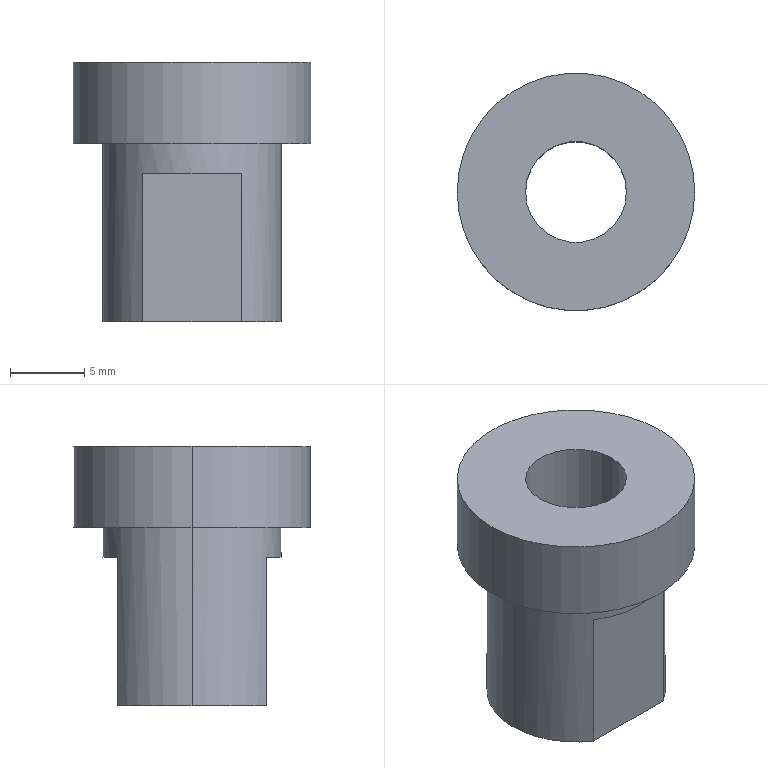Part | STEP file | 2029 Bag feed cylinder joint | 1 solid | 13 faces | box 16 x 16 x 17.5 mm | volume 1737 mm3 | plane 7 | cylinder 6 | commonest cylinder face diameters 6.8 x2 12 x2 16 x2
STEP:
#1=CARTESIAN_POINT('',(0.,0.,0.));
#2=DIRECTION('',(0.,0.,1.));
#3=DIRECTION('',(1.,0.,0.));
#4=AXIS2_PLACEMENT_3D('',#1,#2,#3);
#5=CARTESIAN_POINT('',(-3.4,0.,17.5));
#6=VERTEX_POINT('',#5);
#7=CARTESIAN_POINT('',(-3.4,0.,0.));
#8=VERTEX_POINT('',#7);
#9=CARTESIAN_POINT('',(-3.4,0.,0.));
#10=DIRECTION('',(0.,0.,-1.));
#11=VECTOR('',#10,1.);
#12=LINE('',#9,#11);
#13=CARTESIAN_POINT('',(0.,0.,0.));
#14=DIRECTION('',(0.,0.,-1.));
#15=DIRECTION('',(-1.,0.,0.));
#16=AXIS2_PLACEMENT_3D('',#13,#14,#15);
#17=CYLINDRICAL_SURFACE('',#16,3.4);
#18=CARTESIAN_POINT('',(6.283,0.));
#19=DIRECTION('',(0.,1.));
#20=VECTOR('',#19,1.);
#21=LINE('',#18,#20);
#22=(GEOMETRIC_REPRESENTATION_CONTEXT(2)PARAMETRIC_REPRESENTATION_CONTEXT()REPRESENTATION_CONTEXT('',''));
#23=DEFINITIONAL_REPRESENTATION('',(#21),#22);
#24=PCURVE('',#17,#23);
#25=CARTESIAN_POINT('',(0.,0.,0.));
#26=DIRECTION('',(0.,0.,-1.));
#27=DIRECTION('',(-1.,0.,0.));
#28=AXIS2_PLACEMENT_3D('',#25,#26,#27);
#29=CYLINDRICAL_SURFACE('',#28,3.4);
#30=CARTESIAN_POINT('',(0.,0.));
#31=DIRECTION('',(0.,1.));
#32=VECTOR('',#31,1.);
#33=LINE('',#30,#32);
#34=(GEOMETRIC_REPRESENTATION_CONTEXT(2)PARAMETRIC_REPRESENTATION_CONTEXT()REPRESENTATION_CONTEXT('',''));
#35=DEFINITIONAL_REPRESENTATION('',(#33),#34);
#36=PCURVE('',#29,#35);
#37=SURFACE_CURVE('',#12,(#24,#36),.PCURVE_S1.);
#38=EDGE_CURVE('',#6,#8,#37,.T.);
#39=ORIENTED_EDGE('',*,*,#38,.T.);
#40=CARTESIAN_POINT('',(3.4,0.,0.));
#41=VERTEX_POINT('',#40);
#42=CARTESIAN_POINT('',(0.,0.,0.));
#43=DIRECTION('',(0.,0.,-1.));
#44=DIRECTION('',(-1.,0.,0.));
#45=AXIS2_PLACEMENT_3D('',#42,#43,#44);
#46=CIRCLE('',#45,3.4);
#47=CARTESIAN_POINT('',(0.,0.));
#48=DIRECTION('',(1.,0.));
#49=VECTOR('',#48,1.);
#50=LINE('',#47,#49);
#51=(GEOMETRIC_REPRESENTATION_CONTEXT(2)PARAMETRIC_REPRESENTATION_CONTEXT()REPRESENTATION_CONTEXT('',''));
#52=DEFINITIONAL_REPRESENTATION('',(#50),#51);
#53=PCURVE('',#17,#52);
#54=CARTESIAN_POINT('',(0.,0.,0.));
#55=DIRECTION('',(0.,0.,1.));
#56=DIRECTION('',(1.,0.,0.));
#57=AXIS2_PLACEMENT_3D('',#54,#55,#56);
#58=PLANE('',#57);
#59=CARTESIAN_POINT('',(-3.4,0.));
#60=CARTESIAN_POINT('',(-3.4,5.889));
#61=CARTESIAN_POINT('',(1.7,2.944));
#62=CARTESIAN_POINT('',(6.8,0.));
#63=CARTESIAN_POINT('',(1.7,-2.944));
#64=CARTESIAN_POINT('',(-3.4,-5.889));
#65=CARTESIAN_POINT('',(-3.4,0.));
#66=(BOUNDED_CURVE()B_SPLINE_CURVE(2,(#59,#60,#61,#62,#63,#64,#65),.UNSPECIFIED.,.T.,.F.)B_SPLINE_CURVE_WITH_KNOTS((1,2,2,2,2,1),(-2.094,0.,2.094,4.189,6.283,8.378),.UNSPECIFIED.)CURVE()GEOMETRIC_REPRESENTATION_ITEM()RATIONAL_B_SPLINE_CURVE((1.,0.5,1.,0.5,1.,0.5,1.))REPRESENTATION_ITEM(''));
#67=(GEOMETRIC_REPRESENTATION_CONTEXT(2)PARAMETRIC_REPRESENTATION_CONTEXT()REPRESENTATION_CONTEXT('',''));
#68=DEFINITIONAL_REPRESENTATION('',(#66),#67);
#69=PCURVE('',#58,#68);
#70=SURFACE_CURVE('',#46,(#53,#69),.PCURVE_S1.);
#71=EDGE_CURVE('',#41,#8,#70,.T.);
#72=ORIENTED_EDGE('',*,*,#71,.F.);
#73=CARTESIAN_POINT('',(3.4,0.,17.5));
#74=VERTEX_POINT('',#73);
#75=CARTESIAN_POINT('',(3.4,0.,0.));
#76=DIRECTION('',(0.,0.,-1.));
#77=VECTOR('',#76,1.);
#78=LINE('',#75,#77);
#79=CARTESIAN_POINT('',(3.142,0.));
#80=DIRECTION('',(0.,1.));
#81=VECTOR('',#80,1.);
#82=LINE('',#79,#81);
#83=(GEOMETRIC_REPRESENTATION_CONTEXT(2)PARAMETRIC_REPRESENTATION_CONTEXT()REPRESENTATION_CONTEXT('',''));
#84=DEFINITIONAL_REPRESENTATION('',(#82),#83);
#85=PCURVE('',#17,#84);
#86=CARTESIAN_POINT('',(3.142,0.));
#87=DIRECTION('',(0.,1.));
#88=VECTOR('',#87,1.);
#89=LINE('',#86,#88);
#90=(GEOMETRIC_REPRESENTATION_CONTEXT(2)PARAMETRIC_REPRESENTATION_CONTEXT()REPRESENTATION_CONTEXT('',''));
#91=DEFINITIONAL_REPRESENTATION('',(#89),#90);
#92=PCURVE('',#29,#91);
#93=SURFACE_CURVE('',#78,(#85,#92),.PCURVE_S1.);
#94=EDGE_CURVE('',#74,#41,#93,.T.);
#95=ORIENTED_EDGE('',*,*,#94,.F.);
#96=CARTESIAN_POINT('',(0.,0.,17.5));
#97=DIRECTION('',(0.,0.,-1.));
#98=DIRECTION('',(-1.,0.,0.));
#99=AXIS2_PLACEMENT_3D('',#96,#97,#98);
#100=CIRCLE('',#99,3.4);
#101=CARTESIAN_POINT('',(0.,-17.5));
#102=DIRECTION('',(1.,0.));
#103=VECTOR('',#102,1.);
#104=LINE('',#101,#103);
#105=(GEOMETRIC_REPRESENTATION_CONTEXT(2)PARAMETRIC_REPRESENTATION_CONTEXT()REPRESENTATION_CONTEXT('',''));
#106=DEFINITIONAL_REPRESENTATION('',(#104),#105);
#107=PCURVE('',#17,#106);
#108=CARTESIAN_POINT('',(0.,0.,17.5));
#109=DIRECTION('',(0.,0.,1.));
#110=DIRECTION('',(1.,0.,0.));
#111=AXIS2_PLACEMENT_3D('',#108,#109,#110);
#112=PLANE('',#111);
#113=CARTESIAN_POINT('',(-3.4,0.));
#114=CARTESIAN_POINT('',(-3.4,5.889));
#115=CARTESIAN_POINT('',(1.7,2.944));
#116=CARTESIAN_POINT('',(6.8,0.));
#117=CARTESIAN_POINT('',(1.7,-2.944));
#118=CARTESIAN_POINT('',(-3.4,-5.889));
#119=CARTESIAN_POINT('',(-3.4,0.));
#120=(BOUNDED_CURVE()B_SPLINE_CURVE(2,(#113,#114,#115,#116,#117,#118,#119),.UNSPECIFIED.,.T.,.F.)B_SPLINE_CURVE_WITH_KNOTS((1,2,2,2,2,1),(-2.094,0.,2.094,4.189,6.283,8.378),.UNSPECIFIED.)CURVE()GEOMETRIC_REPRESENTATION_ITEM()RATIONAL_B_SPLINE_CURVE((1.,0.5,1.,0.5,1.,0.5,1.))REPRESENTATION_ITEM(''));
#121=(GEOMETRIC_REPRESENTATION_CONTEXT(2)PARAMETRIC_REPRESENTATION_CONTEXT()REPRESENTATION_CONTEXT('',''));
#122=DEFINITIONAL_REPRESENTATION('',(#120),#121);
#123=PCURVE('',#112,#122);
#124=SURFACE_CURVE('',#100,(#107,#123),.PCURVE_S1.);
#125=EDGE_CURVE('',#74,#6,#124,.T.);
#126=ORIENTED_EDGE('',*,*,#125,.T.);
#127=EDGE_LOOP('',(#39,#72,#95,#126));
#128=FACE_BOUND('',#127,.F.);
#129=ADVANCED_FACE('',(#128),#17,.F.);
#130=CARTESIAN_POINT('',(8.,0.,17.5));
#131=VERTEX_POINT('',#130);
#132=CARTESIAN_POINT('',(-8.,0.,17.5));
#133=VERTEX_POINT('',#132);
#134=CARTESIAN_POINT('',(0.,0.,17.5));
#135=DIRECTION('',(0.,0.,1.));
#136=DIRECTION('',(1.,0.,0.));
#137=AXIS2_PLACEMENT_3D('',#134,#135,#136);
#138=CIRCLE('',#137,8.);
#139=CARTESIAN_POINT('',(0.,0.,17.5));
#140=DIRECTION('',(0.,0.,-1.));
#141=DIRECTION('',(-1.,0.,0.));
#142=AXIS2_PLACEMENT_3D('',#139,#140,#141);
#143=CYLINDRICAL_SURFACE('',#142,8.);
#144=CARTESIAN_POINT('',(3.142,0.));
#145=DIRECTION('',(-1.,0.));
#146=VECTOR('',#145,1.);
#147=LINE('',#144,#146);
#148=(GEOMETRIC_REPRESENTATION_CONTEXT(2)PARAMETRIC_REPRESENTATION_CONTEXT()REPRESENTATION_CONTEXT('',''));
#149=DEFINITIONAL_REPRESENTATION('',(#147),#148);
#150=PCURVE('',#143,#149);
#151=CARTESIAN_POINT('',(0.,0.));
#152=DIRECTION('',(1.,0.));
#153=AXIS2_PLACEMENT_2D('',#151,#152);
#154=CIRCLE('',#153,8.);
#155=(GEOMETRIC_REPRESENTATION_CONTEXT(2)PARAMETRIC_REPRESENTATION_CONTEXT()REPRESENTATION_CONTEXT('',''));
#156=DEFINITIONAL_REPRESENTATION('',(#154),#155);
#157=PCURVE('',#112,#156);
#158=SURFACE_CURVE('',#138,(#150,#157),.PCURVE_S1.);
#159=EDGE_CURVE('',#131,#133,#158,.T.);
#160=ORIENTED_EDGE('',*,*,#159,.F.);
#161=CARTESIAN_POINT('',(8.,0.,12.));
#162=VERTEX_POINT('',#161);
#163=CARTESIAN_POINT('',(8.,0.,17.5));
#164=DIRECTION('',(0.,0.,-1.));
#165=VECTOR('',#164,1.);
#166=LINE('',#163,#165);
#167=CARTESIAN_POINT('',(3.142,0.));
#168=DIRECTION('',(0.,1.));
#169=VECTOR('',#168,1.);
#170=LINE('',#167,#169);
#171=(GEOMETRIC_REPRESENTATION_CONTEXT(2)PARAMETRIC_REPRESENTATION_CONTEXT()REPRESENTATION_CONTEXT('',''));
#172=DEFINITIONAL_REPRESENTATION('',(#170),#171);
#173=PCURVE('',#143,#172);
#174=CARTESIAN_POINT('',(0.,0.,17.5));
#175=DIRECTION('',(0.,0.,-1.));
#176=DIRECTION('',(-1.,0.,0.));
#177=AXIS2_PLACEMENT_3D('',#174,#175,#176);
#178=CYLINDRICAL_SURFACE('',#177,8.);
#179=CARTESIAN_POINT('',(3.142,0.));
#180=DIRECTION('',(0.,1.));
#181=VECTOR('',#180,1.);
#182=LINE('',#179,#181);
#183=(GEOMETRIC_REPRESENTATION_CONTEXT(2)PARAMETRIC_REPRESENTATION_CONTEXT()REPRESENTATION_CONTEXT('',''));
#184=DEFINITIONAL_REPRESENTATION('',(#182),#183);
#185=PCURVE('',#178,#184);
#186=SURFACE_CURVE('',#166,(#173,#185),.PCURVE_S1.);
#187=EDGE_CURVE('',#131,#162,#186,.T.);
#188=ORIENTED_EDGE('',*,*,#187,.T.);
#189=CARTESIAN_POINT('',(-8.,0.,12.));
#190=VERTEX_POINT('',#189);
#191=CARTESIAN_POINT('',(0.,0.,12.));
#192=DIRECTION('',(0.,0.,1.));
#193=DIRECTION('',(1.,0.,0.));
#194=AXIS2_PLACEMENT_3D('',#191,#192,#193);
#195=CIRCLE('',#194,8.);
#196=CARTESIAN_POINT('',(3.142,5.5));
#197=DIRECTION('',(-1.,0.));
#198=VECTOR('',#197,1.);
#199=LINE('',#196,#198);
#200=(GEOMETRIC_REPRESENTATION_CONTEXT(2)PARAMETRIC_REPRESENTATION_CONTEXT()REPRESENTATION_CONTEXT('',''));
#201=DEFINITIONAL_REPRESENTATION('',(#199),#200);
#202=PCURVE('',#143,#201);
#203=CARTESIAN_POINT('',(0.,0.,12.));
#204=DIRECTION('',(0.,0.,1.));
#205=DIRECTION('',(1.,0.,0.));
#206=AXIS2_PLACEMENT_3D('',#203,#204,#205);
#207=PLANE('',#206);
#208=CARTESIAN_POINT('',(0.,0.));
#209=DIRECTION('',(1.,0.));
#210=AXIS2_PLACEMENT_2D('',#208,#209);
#211=CIRCLE('',#210,8.);
#212=(GEOMETRIC_REPRESENTATION_CONTEXT(2)PARAMETRIC_REPRESENTATION_CONTEXT()REPRESENTATION_CONTEXT('',''));
#213=DEFINITIONAL_REPRESENTATION('',(#211),#212);
#214=PCURVE('',#207,#213);
#215=SURFACE_CURVE('',#195,(#202,#214),.PCURVE_S1.);
#216=EDGE_CURVE('',#162,#190,#215,.T.);
#217=ORIENTED_EDGE('',*,*,#216,.T.);
#218=CARTESIAN_POINT('',(-8.,0.,17.5));
#219=DIRECTION('',(0.,0.,-1.));
#220=VECTOR('',#219,1.);
#221=LINE('',#218,#220);
#222=CARTESIAN_POINT('',(0.,0.));
#223=DIRECTION('',(0.,1.));
#224=VECTOR('',#223,1.);
#225=LINE('',#222,#224);
#226=(GEOMETRIC_REPRESENTATION_CONTEXT(2)PARAMETRIC_REPRESENTATION_CONTEXT()REPRESENTATION_CONTEXT('',''));
#227=DEFINITIONAL_REPRESENTATION('',(#225),#226);
#228=PCURVE('',#143,#227);
#229=CARTESIAN_POINT('',(6.283,0.));
#230=DIRECTION('',(0.,1.));
#231=VECTOR('',#230,1.);
#232=LINE('',#229,#231);
#233=(GEOMETRIC_REPRESENTATION_CONTEXT(2)PARAMETRIC_REPRESENTATION_CONTEXT()REPRESENTATION_CONTEXT('',''));
#234=DEFINITIONAL_REPRESENTATION('',(#232),#233);
#235=PCURVE('',#178,#234);
#236=SURFACE_CURVE('',#221,(#228,#235),.PCURVE_S1.);
#237=EDGE_CURVE('',#133,#190,#236,.T.);
#238=ORIENTED_EDGE('',*,*,#237,.F.);
#239=EDGE_LOOP('',(#160,#188,#217,#238));
#240=FACE_BOUND('',#239,.T.);
#241=ADVANCED_FACE('',(#240),#143,.T.);
#242=CARTESIAN_POINT('',(6.,0.,12.));
#243=VERTEX_POINT('',#242);
#244=CARTESIAN_POINT('',(-6.,0.,12.));
#245=VERTEX_POINT('',#244);
#246=CARTESIAN_POINT('',(0.,0.,12.));
#247=DIRECTION('',(0.,0.,1.));
#248=DIRECTION('',(1.,0.,0.));
#249=AXIS2_PLACEMENT_3D('',#246,#247,#248);
#250=CIRCLE('',#249,6.);
#251=CARTESIAN_POINT('',(0.,0.,12.));
#252=DIRECTION('',(0.,0.,-1.));
#253=DIRECTION('',(-1.,0.,0.));
#254=AXIS2_PLACEMENT_3D('',#251,#252,#253);
#255=CYLINDRICAL_SURFACE('',#254,6.);
#256=CARTESIAN_POINT('',(3.142,0.));
#257=DIRECTION('',(-1.,0.));
#258=VECTOR('',#257,1.);
#259=LINE('',#256,#258);
#260=(GEOMETRIC_REPRESENTATION_CONTEXT(2)PARAMETRIC_REPRESENTATION_CONTEXT()REPRESENTATION_CONTEXT('',''));
#261=DEFINITIONAL_REPRESENTATION('',(#259),#260);
#262=PCURVE('',#255,#261);
#263=CARTESIAN_POINT('',(0.,0.));
#264=DIRECTION('',(1.,0.));
#265=AXIS2_PLACEMENT_2D('',#263,#264);
#266=CIRCLE('',#265,6.);
#267=(GEOMETRIC_REPRESENTATION_CONTEXT(2)PARAMETRIC_REPRESENTATION_CONTEXT()REPRESENTATION_CONTEXT('',''));
#268=DEFINITIONAL_REPRESENTATION('',(#266),#267);
#269=PCURVE('',#207,#268);
#270=SURFACE_CURVE('',#250,(#262,#269),.PCURVE_S1.);
#271=EDGE_CURVE('',#243,#245,#270,.T.);
#272=ORIENTED_EDGE('',*,*,#271,.F.);
#273=CARTESIAN_POINT('',(6.,0.,0.));
#274=VERTEX_POINT('',#273);
#275=CARTESIAN_POINT('',(6.,0.,12.));
#276=DIRECTION('',(0.,0.,-1.));
#277=VECTOR('',#276,1.);
#278=LINE('',#275,#277);
#279=CARTESIAN_POINT('',(3.142,0.));
#280=DIRECTION('',(0.,1.));
#281=VECTOR('',#280,1.);
#282=LINE('',#279,#281);
#283=(GEOMETRIC_REPRESENTATION_CONTEXT(2)PARAMETRIC_REPRESENTATION_CONTEXT()REPRESENTATION_CONTEXT('',''));
#284=DEFINITIONAL_REPRESENTATION('',(#282),#283);
#285=PCURVE('',#255,#284);
#286=CARTESIAN_POINT('',(0.,0.,12.));
#287=DIRECTION('',(0.,0.,-1.));
#288=DIRECTION('',(-1.,0.,0.));
#289=AXIS2_PLACEMENT_3D('',#286,#287,#288);
#290=CYLINDRICAL_SURFACE('',#289,6.);
#291=CARTESIAN_POINT('',(3.142,0.));
#292=DIRECTION('',(0.,1.));
#293=VECTOR('',#292,1.);
#294=LINE('',#291,#293);
#295=(GEOMETRIC_REPRESENTATION_CONTEXT(2)PARAMETRIC_REPRESENTATION_CONTEXT()REPRESENTATION_CONTEXT('',''));
#296=DEFINITIONAL_REPRESENTATION('',(#294),#295);
#297=PCURVE('',#290,#296);
#298=SURFACE_CURVE('',#278,(#285,#297),.PCURVE_S1.);
#299=EDGE_CURVE('',#243,#274,#298,.T.);
#300=ORIENTED_EDGE('',*,*,#299,.T.);
#301=CARTESIAN_POINT('',(3.317,5.,0.));
#302=VERTEX_POINT('',#301);
#303=CARTESIAN_POINT('',(0.,0.,0.));
#304=DIRECTION('',(0.,0.,1.));
#305=DIRECTION('',(1.,0.,0.));
#306=AXIS2_PLACEMENT_3D('',#303,#304,#305);
#307=CIRCLE('',#306,6.);
#308=CARTESIAN_POINT('',(3.142,12.));
#309=DIRECTION('',(-1.,0.));
#310=VECTOR('',#309,1.);
#311=LINE('',#308,#310);
#312=(GEOMETRIC_REPRESENTATION_CONTEXT(2)PARAMETRIC_REPRESENTATION_CONTEXT()REPRESENTATION_CONTEXT('',''));
#313=DEFINITIONAL_REPRESENTATION('',(#311),#312);
#314=PCURVE('',#255,#313);
#315=CARTESIAN_POINT('',(0.,0.));
#316=DIRECTION('',(1.,0.));
#317=AXIS2_PLACEMENT_2D('',#315,#316);
#318=CIRCLE('',#317,6.);
#319=(GEOMETRIC_REPRESENTATION_CONTEXT(2)PARAMETRIC_REPRESENTATION_CONTEXT()REPRESENTATION_CONTEXT('',''));
#320=DEFINITIONAL_REPRESENTATION('',(#318),#319);
#321=PCURVE('',#58,#320);
#322=SURFACE_CURVE('',#307,(#314,#321),.PCURVE_S1.);
#323=EDGE_CURVE('',#274,#302,#322,.T.);
#324=ORIENTED_EDGE('',*,*,#323,.T.);
#325=CARTESIAN_POINT('',(3.317,5.,10.));
#326=VERTEX_POINT('',#325);
#327=CARTESIAN_POINT('',(3.317,5.,12.));
#328=DIRECTION('',(0.,0.,1.));
#329=VECTOR('',#328,1.);
#330=LINE('',#327,#329);
#331=CARTESIAN_POINT('',(2.156,0.));
#332=DIRECTION('',(0.,-1.));
#333=VECTOR('',#332,1.);
#334=LINE('',#331,#333);
#335=(GEOMETRIC_REPRESENTATION_CONTEXT(2)PARAMETRIC_REPRESENTATION_CONTEXT()REPRESENTATION_CONTEXT('',''));
#336=DEFINITIONAL_REPRESENTATION('',(#334),#335);
#337=PCURVE('',#255,#336);
#338=CARTESIAN_POINT('',(6.003,5.,10.));
#339=DIRECTION('',(0.,-1.,0.));
#340=DIRECTION('',(0.,0.,-1.));
#341=AXIS2_PLACEMENT_3D('',#338,#339,#340);
#342=PLANE('',#341);
#343=CARTESIAN_POINT('',(-2.,-2.687));
#344=DIRECTION('',(-1.,0.));
#345=VECTOR('',#344,1.);
#346=LINE('',#343,#345);
#347=(GEOMETRIC_REPRESENTATION_CONTEXT(2)PARAMETRIC_REPRESENTATION_CONTEXT()REPRESENTATION_CONTEXT('',''));
#348=DEFINITIONAL_REPRESENTATION('',(#346),#347);
#349=PCURVE('',#342,#348);
#350=SURFACE_CURVE('',#330,(#337,#349),.PCURVE_S1.);
#351=EDGE_CURVE('',#302,#326,#350,.T.);
#352=ORIENTED_EDGE('',*,*,#351,.T.);
#353=CARTESIAN_POINT('',(-3.317,5.,10.));
#354=VERTEX_POINT('',#353);
#355=CARTESIAN_POINT('',(0.,0.,10.));
#356=DIRECTION('',(0.,0.,-1.));
#357=DIRECTION('',(-1.,0.,0.));
#358=AXIS2_PLACEMENT_3D('',#355,#356,#357);
#359=CIRCLE('',#358,6.);
#360=CARTESIAN_POINT('',(0.,2.));
#361=DIRECTION('',(1.,0.));
#362=VECTOR('',#361,1.);
#363=LINE('',#360,#362);
#364=(GEOMETRIC_REPRESENTATION_CONTEXT(2)PARAMETRIC_REPRESENTATION_CONTEXT()REPRESENTATION_CONTEXT('',''));
#365=DEFINITIONAL_REPRESENTATION('',(#363),#364);
#366=PCURVE('',#255,#365);
#367=CARTESIAN_POINT('',(0.,0.,10.));
#368=DIRECTION('',(0.,0.,-1.));
#369=DIRECTION('',(-1.,0.,0.));
#370=AXIS2_PLACEMENT_3D('',#367,#368,#369);
#371=PLANE('',#370);
#372=CARTESIAN_POINT('',(0.,0.));
#373=DIRECTION('',(1.,0.));
#374=AXIS2_PLACEMENT_2D('',#372,#373);
#375=CIRCLE('',#374,6.);
#376=(GEOMETRIC_REPRESENTATION_CONTEXT(2)PARAMETRIC_REPRESENTATION_CONTEXT()REPRESENTATION_CONTEXT('',''));
#377=DEFINITIONAL_REPRESENTATION('',(#375),#376);
#378=PCURVE('',#371,#377);
#379=SURFACE_CURVE('',#359,(#366,#378),.PCURVE_S1.);
#380=EDGE_CURVE('',#354,#326,#379,.T.);
#381=ORIENTED_EDGE('',*,*,#380,.F.);
#382=CARTESIAN_POINT('',(-3.317,5.,0.));
#383=VERTEX_POINT('',#382);
#384=CARTESIAN_POINT('',(-3.317,5.,12.));
#385=DIRECTION('',(0.,0.,-1.));
#386=VECTOR('',#385,1.);
#387=LINE('',#384,#386);
#388=CARTESIAN_POINT('',(0.9851,0.));
#389=DIRECTION('',(0.,1.));
#390=VECTOR('',#389,1.);
#391=LINE('',#388,#390);
#392=(GEOMETRIC_REPRESENTATION_CONTEXT(2)PARAMETRIC_REPRESENTATION_CONTEXT()REPRESENTATION_CONTEXT('',''));
#393=DEFINITIONAL_REPRESENTATION('',(#391),#392);
#394=PCURVE('',#255,#393);
#395=CARTESIAN_POINT('',(-2.,-9.32));
#396=DIRECTION('',(1.,0.));
#397=VECTOR('',#396,1.);
#398=LINE('',#395,#397);
#399=(GEOMETRIC_REPRESENTATION_CONTEXT(2)PARAMETRIC_REPRESENTATION_CONTEXT()REPRESENTATION_CONTEXT('',''));
#400=DEFINITIONAL_REPRESENTATION('',(#398),#399);
#401=PCURVE('',#342,#400);
#402=SURFACE_CURVE('',#387,(#394,#401),.PCURVE_S1.);
#403=EDGE_CURVE('',#354,#383,#402,.T.);
#404=ORIENTED_EDGE('',*,*,#403,.T.);
#405=CARTESIAN_POINT('',(-6.,0.,0.));
#406=VERTEX_POINT('',#405);
#407=CARTESIAN_POINT('',(0.,0.,0.));
#408=DIRECTION('',(0.,0.,1.));
#409=DIRECTION('',(1.,0.,0.));
#410=AXIS2_PLACEMENT_3D('',#407,#408,#409);
#411=CIRCLE('',#410,6.);
#412=CARTESIAN_POINT('',(3.142,12.));
#413=DIRECTION('',(-1.,0.));
#414=VECTOR('',#413,1.);
#415=LINE('',#412,#414);
#416=(GEOMETRIC_REPRESENTATION_CONTEXT(2)PARAMETRIC_REPRESENTATION_CONTEXT()REPRESENTATION_CONTEXT('',''));
#417=DEFINITIONAL_REPRESENTATION('',(#415),#416);
#418=PCURVE('',#255,#417);
#419=CARTESIAN_POINT('',(0.,0.));
#420=DIRECTION('',(1.,0.));
#421=AXIS2_PLACEMENT_2D('',#419,#420);
#422=CIRCLE('',#421,6.);
#423=(GEOMETRIC_REPRESENTATION_CONTEXT(2)PARAMETRIC_REPRESENTATION_CONTEXT()REPRESENTATION_CONTEXT('',''));
#424=DEFINITIONAL_REPRESENTATION('',(#422),#423);
#425=PCURVE('',#58,#424);
#426=SURFACE_CURVE('',#411,(#418,#425),.PCURVE_S1.);
#427=EDGE_CURVE('',#383,#406,#426,.T.);
#428=ORIENTED_EDGE('',*,*,#427,.T.);
#429=CARTESIAN_POINT('',(-6.,0.,12.));
#430=DIRECTION('',(0.,0.,-1.));
#431=VECTOR('',#430,1.);
#432=LINE('',#429,#431);
#433=CARTESIAN_POINT('',(0.,0.));
#434=DIRECTION('',(0.,1.));
#435=VECTOR('',#434,1.);
#436=LINE('',#433,#435);
#437=(GEOMETRIC_REPRESENTATION_CONTEXT(2)PARAMETRIC_REPRESENTATION_CONTEXT()REPRESENTATION_CONTEXT('',''));
#438=DEFINITIONAL_REPRESENTATION('',(#436),#437);
#439=PCURVE('',#255,#438);
#440=CARTESIAN_POINT('',(6.283,0.));
#441=DIRECTION('',(0.,1.));
#442=VECTOR('',#441,1.);
#443=LINE('',#440,#442);
#444=(GEOMETRIC_REPRESENTATION_CONTEXT(2)PARAMETRIC_REPRESENTATION_CONTEXT()REPRESENTATION_CONTEXT('',''));
#445=DEFINITIONAL_REPRESENTATION('',(#443),#444);
#446=PCURVE('',#290,#445);
#447=SURFACE_CURVE('',#432,(#439,#446),.PCURVE_S1.);
#448=EDGE_CURVE('',#245,#406,#447,.T.);
#449=ORIENTED_EDGE('',*,*,#448,.F.);
#450=EDGE_LOOP('',(#272,#300,#324,#352,#381,#404,#428,#449));
#451=FACE_BOUND('',#450,.T.);
#452=ADVANCED_FACE('',(#451),#255,.T.);
#453=CARTESIAN_POINT('',(0.,0.,17.5));
#454=DIRECTION('',(0.,0.,1.));
#455=DIRECTION('',(1.,0.,0.));
#456=AXIS2_PLACEMENT_3D('',#453,#454,#455);
#457=CIRCLE('',#456,8.);
#458=CARTESIAN_POINT('',(0.,0.));
#459=DIRECTION('',(1.,0.));
#460=AXIS2_PLACEMENT_2D('',#458,#459);
#461=CIRCLE('',#460,8.);
#462=(GEOMETRIC_REPRESENTATION_CONTEXT(2)PARAMETRIC_REPRESENTATION_CONTEXT()REPRESENTATION_CONTEXT('',''));
#463=DEFINITIONAL_REPRESENTATION('',(#461),#462);
#464=PCURVE('',#112,#463);
#465=CARTESIAN_POINT('',(9.425,0.));
#466=DIRECTION('',(-1.,0.));
#467=VECTOR('',#466,1.);
#468=LINE('',#465,#467);
#469=(GEOMETRIC_REPRESENTATION_CONTEXT(2)PARAMETRIC_REPRESENTATION_CONTEXT()REPRESENTATION_CONTEXT('',''));
#470=DEFINITIONAL_REPRESENTATION('',(#468),#469);
#471=PCURVE('',#178,#470);
#472=SURFACE_CURVE('',#457,(#464,#471),.PCURVE_S1.);
#473=EDGE_CURVE('',#133,#131,#472,.T.);
#474=ORIENTED_EDGE('',*,*,#473,.T.);
#475=ORIENTED_EDGE('',*,*,#159,.T.);
#476=EDGE_LOOP('',(#474,#475));
#477=FACE_BOUND('',#476,.T.);
#478=CARTESIAN_POINT('',(0.,0.,17.5));
#479=DIRECTION('',(0.,0.,-1.));
#480=DIRECTION('',(-1.,0.,0.));
#481=AXIS2_PLACEMENT_3D('',#478,#479,#480);
#482=CIRCLE('',#481,3.4);
#483=CARTESIAN_POINT('',(-3.4,0.));
#484=CARTESIAN_POINT('',(-3.4,5.889));
#485=CARTESIAN_POINT('',(1.7,2.944));
#486=CARTESIAN_POINT('',(6.8,0.));
#487=CARTESIAN_POINT('',(1.7,-2.944));
#488=CARTESIAN_POINT('',(-3.4,-5.889));
#489=CARTESIAN_POINT('',(-3.4,0.));
#490=(BOUNDED_CURVE()B_SPLINE_CURVE(2,(#483,#484,#485,#486,#487,#488,#489),.UNSPECIFIED.,.T.,.F.)B_SPLINE_CURVE_WITH_KNOTS((1,2,2,2,2,1),(-2.094,0.,2.094,4.189,6.283,8.378),.UNSPECIFIED.)CURVE()GEOMETRIC_REPRESENTATION_ITEM()RATIONAL_B_SPLINE_CURVE((1.,0.5,1.,0.5,1.,0.5,1.))REPRESENTATION_ITEM(''));
#491=(GEOMETRIC_REPRESENTATION_CONTEXT(2)PARAMETRIC_REPRESENTATION_CONTEXT()REPRESENTATION_CONTEXT('',''));
#492=DEFINITIONAL_REPRESENTATION('',(#490),#491);
#493=PCURVE('',#112,#492);
#494=CARTESIAN_POINT('',(0.,-17.5));
#495=DIRECTION('',(1.,0.));
#496=VECTOR('',#495,1.);
#497=LINE('',#494,#496);
#498=(GEOMETRIC_REPRESENTATION_CONTEXT(2)PARAMETRIC_REPRESENTATION_CONTEXT()REPRESENTATION_CONTEXT('',''));
#499=DEFINITIONAL_REPRESENTATION('',(#497),#498);
#500=PCURVE('',#29,#499);
#501=SURFACE_CURVE('',#482,(#493,#500),.PCURVE_S1.);
#502=EDGE_CURVE('',#6,#74,#501,.T.);
#503=ORIENTED_EDGE('',*,*,#502,.T.);
#504=ORIENTED_EDGE('',*,*,#125,.T.);
#505=EDGE_LOOP('',(#503,#504));
#506=FACE_BOUND('',#505,.T.);
#507=ADVANCED_FACE('',(#477,#506),#112,.T.);
#508=ORIENTED_EDGE('',*,*,#299,.F.);
#509=CARTESIAN_POINT('',(0.,0.,12.));
#510=DIRECTION('',(0.,0.,1.));
#511=DIRECTION('',(1.,0.,0.));
#512=AXIS2_PLACEMENT_3D('',#509,#510,#511);
#513=CIRCLE('',#512,6.);
#514=CARTESIAN_POINT('',(9.425,0.));
#515=DIRECTION('',(-1.,0.));
#516=VECTOR('',#515,1.);
#517=LINE('',#514,#516);
#518=(GEOMETRIC_REPRESENTATION_CONTEXT(2)PARAMETRIC_REPRESENTATION_CONTEXT()REPRESENTATION_CONTEXT('',''));
#519=DEFINITIONAL_REPRESENTATION('',(#517),#518);
#520=PCURVE('',#290,#519);
#521=CARTESIAN_POINT('',(0.,0.));
#522=DIRECTION('',(1.,0.));
#523=AXIS2_PLACEMENT_2D('',#521,#522);
#524=CIRCLE('',#523,6.);
#525=(GEOMETRIC_REPRESENTATION_CONTEXT(2)PARAMETRIC_REPRESENTATION_CONTEXT()REPRESENTATION_CONTEXT('',''));
#526=DEFINITIONAL_REPRESENTATION('',(#524),#525);
#527=PCURVE('',#207,#526);
#528=SURFACE_CURVE('',#513,(#520,#527),.PCURVE_S1.);
#529=EDGE_CURVE('',#245,#243,#528,.T.);
#530=ORIENTED_EDGE('',*,*,#529,.F.);
#531=ORIENTED_EDGE('',*,*,#448,.T.);
#532=CARTESIAN_POINT('',(-3.317,-5.,0.));
#533=VERTEX_POINT('',#532);
#534=CARTESIAN_POINT('',(0.,0.,0.));
#535=DIRECTION('',(0.,0.,1.));
#536=DIRECTION('',(1.,0.,0.));
#537=AXIS2_PLACEMENT_3D('',#534,#535,#536);
#538=CIRCLE('',#537,6.);
#539=CARTESIAN_POINT('',(9.425,12.));
#540=DIRECTION('',(-1.,0.));
#541=VECTOR('',#540,1.);
#542=LINE('',#539,#541);
#543=(GEOMETRIC_REPRESENTATION_CONTEXT(2)PARAMETRIC_REPRESENTATION_CONTEXT()REPRESENTATION_CONTEXT('',''));
#544=DEFINITIONAL_REPRESENTATION('',(#542),#543);
#545=PCURVE('',#290,#544);
#546=CARTESIAN_POINT('',(0.,0.));
#547=DIRECTION('',(1.,0.));
#548=AXIS2_PLACEMENT_2D('',#546,#547);
#549=CIRCLE('',#548,6.);
#550=(GEOMETRIC_REPRESENTATION_CONTEXT(2)PARAMETRIC_REPRESENTATION_CONTEXT()REPRESENTATION_CONTEXT('',''));
#551=DEFINITIONAL_REPRESENTATION('',(#549),#550);
#552=PCURVE('',#58,#551);
#553=SURFACE_CURVE('',#538,(#545,#552),.PCURVE_S1.);
#554=EDGE_CURVE('',#406,#533,#553,.T.);
#555=ORIENTED_EDGE('',*,*,#554,.T.);
#556=CARTESIAN_POINT('',(-3.317,-5.,10.));
#557=VERTEX_POINT('',#556);
#558=CARTESIAN_POINT('',(-3.317,-5.,12.));
#559=DIRECTION('',(0.,0.,1.));
#560=VECTOR('',#559,1.);
#561=LINE('',#558,#560);
#562=CARTESIAN_POINT('',(5.298,0.));
#563=DIRECTION('',(0.,-1.));
#564=VECTOR('',#563,1.);
#565=LINE('',#562,#564);
#566=(GEOMETRIC_REPRESENTATION_CONTEXT(2)PARAMETRIC_REPRESENTATION_CONTEXT()REPRESENTATION_CONTEXT('',''));
#567=DEFINITIONAL_REPRESENTATION('',(#565),#566);
#568=PCURVE('',#290,#567);
#569=CARTESIAN_POINT('',(-11.365,-5.,10.));
#570=DIRECTION('',(0.,1.,0.));
#571=DIRECTION('',(-1.,0.,0.));
#572=AXIS2_PLACEMENT_3D('',#569,#570,#571);
#573=PLANE('',#572);
#574=CARTESIAN_POINT('',(-8.049,2.));
#575=DIRECTION('',(0.,1.));
#576=VECTOR('',#575,1.);
#577=LINE('',#574,#576);
#578=(GEOMETRIC_REPRESENTATION_CONTEXT(2)PARAMETRIC_REPRESENTATION_CONTEXT()REPRESENTATION_CONTEXT('',''));
#579=DEFINITIONAL_REPRESENTATION('',(#577),#578);
#580=PCURVE('',#573,#579);
#581=SURFACE_CURVE('',#561,(#568,#580),.PCURVE_S1.);
#582=EDGE_CURVE('',#533,#557,#581,.T.);
#583=ORIENTED_EDGE('',*,*,#582,.T.);
#584=CARTESIAN_POINT('',(3.317,-5.,10.));
#585=VERTEX_POINT('',#584);
#586=CARTESIAN_POINT('',(0.,0.,10.));
#587=DIRECTION('',(0.,0.,-1.));
#588=DIRECTION('',(-1.,0.,0.));
#589=AXIS2_PLACEMENT_3D('',#586,#587,#588);
#590=CIRCLE('',#589,6.);
#591=CARTESIAN_POINT('',(0.,2.));
#592=DIRECTION('',(1.,0.));
#593=VECTOR('',#592,1.);
#594=LINE('',#591,#593);
#595=(GEOMETRIC_REPRESENTATION_CONTEXT(2)PARAMETRIC_REPRESENTATION_CONTEXT()REPRESENTATION_CONTEXT('',''));
#596=DEFINITIONAL_REPRESENTATION('',(#594),#595);
#597=PCURVE('',#290,#596);
#598=CARTESIAN_POINT('',(0.,0.,10.));
#599=DIRECTION('',(0.,0.,-1.));
#600=DIRECTION('',(-1.,0.,0.));
#601=AXIS2_PLACEMENT_3D('',#598,#599,#600);
#602=PLANE('',#601);
#603=CARTESIAN_POINT('',(0.,0.));
#604=DIRECTION('',(1.,0.));
#605=AXIS2_PLACEMENT_2D('',#603,#604);
#606=CIRCLE('',#605,6.);
#607=(GEOMETRIC_REPRESENTATION_CONTEXT(2)PARAMETRIC_REPRESENTATION_CONTEXT()REPRESENTATION_CONTEXT('',''));
#608=DEFINITIONAL_REPRESENTATION('',(#606),#607);
#609=PCURVE('',#602,#608);
#610=SURFACE_CURVE('',#590,(#597,#609),.PCURVE_S1.);
#611=EDGE_CURVE('',#585,#557,#610,.T.);
#612=ORIENTED_EDGE('',*,*,#611,.F.);
#613=CARTESIAN_POINT('',(3.317,-5.,0.));
#614=VERTEX_POINT('',#613);
#615=CARTESIAN_POINT('',(3.317,-5.,12.));
#616=DIRECTION('',(0.,0.,-1.));
#617=VECTOR('',#616,1.);
#618=LINE('',#615,#617);
#619=CARTESIAN_POINT('',(4.127,0.));
#620=DIRECTION('',(0.,1.));
#621=VECTOR('',#620,1.);
#622=LINE('',#619,#621);
#623=(GEOMETRIC_REPRESENTATION_CONTEXT(2)PARAMETRIC_REPRESENTATION_CONTEXT()REPRESENTATION_CONTEXT('',''));
#624=DEFINITIONAL_REPRESENTATION('',(#622),#623);
#625=PCURVE('',#290,#624);
#626=CARTESIAN_POINT('',(-14.682,2.));
#627=DIRECTION('',(0.,-1.));
#628=VECTOR('',#627,1.);
#629=LINE('',#626,#628);
#630=(GEOMETRIC_REPRESENTATION_CONTEXT(2)PARAMETRIC_REPRESENTATION_CONTEXT()REPRESENTATION_CONTEXT('',''));
#631=DEFINITIONAL_REPRESENTATION('',(#629),#630);
#632=PCURVE('',#573,#631);
#633=SURFACE_CURVE('',#618,(#625,#632),.PCURVE_S1.);
#634=EDGE_CURVE('',#585,#614,#633,.T.);
#635=ORIENTED_EDGE('',*,*,#634,.T.);
#636=CARTESIAN_POINT('',(0.,0.,0.));
#637=DIRECTION('',(0.,0.,1.));
#638=DIRECTION('',(1.,0.,0.));
#639=AXIS2_PLACEMENT_3D('',#636,#637,#638);
#640=CIRCLE('',#639,6.);
#641=CARTESIAN_POINT('',(9.425,12.));
#642=DIRECTION('',(-1.,0.));
#643=VECTOR('',#642,1.);
#644=LINE('',#641,#643);
#645=(GEOMETRIC_REPRESENTATION_CONTEXT(2)PARAMETRIC_REPRESENTATION_CONTEXT()REPRESENTATION_CONTEXT('',''));
#646=DEFINITIONAL_REPRESENTATION('',(#644),#645);
#647=PCURVE('',#290,#646);
#648=CARTESIAN_POINT('',(0.,0.));
#649=DIRECTION('',(1.,0.));
#650=AXIS2_PLACEMENT_2D('',#648,#649);
#651=CIRCLE('',#650,6.);
#652=(GEOMETRIC_REPRESENTATION_CONTEXT(2)PARAMETRIC_REPRESENTATION_CONTEXT()REPRESENTATION_CONTEXT('',''));
#653=DEFINITIONAL_REPRESENTATION('',(#651),#652);
#654=PCURVE('',#58,#653);
#655=SURFACE_CURVE('',#640,(#647,#654),.PCURVE_S1.);
#656=EDGE_CURVE('',#614,#274,#655,.T.);
#657=ORIENTED_EDGE('',*,*,#656,.T.);
#658=EDGE_LOOP('',(#508,#530,#531,#555,#583,#612,#635,#657));
#659=FACE_BOUND('',#658,.T.);
#660=ADVANCED_FACE('',(#659),#290,.T.);
#661=CARTESIAN_POINT('',(0.,0.,0.));
#662=DIRECTION('',(0.,0.,-1.));
#663=DIRECTION('',(-1.,0.,0.));
#664=AXIS2_PLACEMENT_3D('',#661,#662,#663);
#665=CIRCLE('',#664,3.4);
#666=CARTESIAN_POINT('',(-3.4,0.));
#667=CARTESIAN_POINT('',(-3.4,5.889));
#668=CARTESIAN_POINT('',(1.7,2.944));
#669=CARTESIAN_POINT('',(6.8,0.));
#670=CARTESIAN_POINT('',(1.7,-2.944));
#671=CARTESIAN_POINT('',(-3.4,-5.889));
#672=CARTESIAN_POINT('',(-3.4,0.));
#673=(BOUNDED_CURVE()B_SPLINE_CURVE(2,(#666,#667,#668,#669,#670,#671,#672),.UNSPECIFIED.,.T.,.F.)B_SPLINE_CURVE_WITH_KNOTS((1,2,2,2,2,1),(-2.094,0.,2.094,4.189,6.283,8.378),.UNSPECIFIED.)CURVE()GEOMETRIC_REPRESENTATION_ITEM()RATIONAL_B_SPLINE_CURVE((1.,0.5,1.,0.5,1.,0.5,1.))REPRESENTATION_ITEM(''));
#674=(GEOMETRIC_REPRESENTATION_CONTEXT(2)PARAMETRIC_REPRESENTATION_CONTEXT()REPRESENTATION_CONTEXT('',''));
#675=DEFINITIONAL_REPRESENTATION('',(#673),#674);
#676=PCURVE('',#58,#675);
#677=CARTESIAN_POINT('',(0.,0.));
#678=DIRECTION('',(1.,0.));
#679=VECTOR('',#678,1.);
#680=LINE('',#677,#679);
#681=(GEOMETRIC_REPRESENTATION_CONTEXT(2)PARAMETRIC_REPRESENTATION_CONTEXT()REPRESENTATION_CONTEXT('',''));
#682=DEFINITIONAL_REPRESENTATION('',(#680),#681);
#683=PCURVE('',#29,#682);
#684=SURFACE_CURVE('',#665,(#676,#683),.PCURVE_S1.);
#685=EDGE_CURVE('',#8,#41,#684,.T.);
#686=ORIENTED_EDGE('',*,*,#685,.F.);
#687=ORIENTED_EDGE('',*,*,#71,.F.);
#688=EDGE_LOOP('',(#686,#687));
#689=FACE_BOUND('',#688,.T.);
#690=ORIENTED_EDGE('',*,*,#656,.F.);
#691=CARTESIAN_POINT('',(0.,-5.,0.));
#692=DIRECTION('',(-1.,0.,0.));
#693=VECTOR('',#692,1.);
#694=LINE('',#691,#693);
#695=CARTESIAN_POINT('',(0.,-5.));
#696=DIRECTION('',(-1.,0.));
#697=VECTOR('',#696,1.);
#698=LINE('',#695,#697);
#699=(GEOMETRIC_REPRESENTATION_CONTEXT(2)PARAMETRIC_REPRESENTATION_CONTEXT()REPRESENTATION_CONTEXT('',''));
#700=DEFINITIONAL_REPRESENTATION('',(#698),#699);
#701=PCURVE('',#58,#700);
#702=CARTESIAN_POINT('',(-11.365,-10.));
#703=DIRECTION('',(1.,0.));
#704=VECTOR('',#703,1.);
#705=LINE('',#702,#704);
#706=(GEOMETRIC_REPRESENTATION_CONTEXT(2)PARAMETRIC_REPRESENTATION_CONTEXT()REPRESENTATION_CONTEXT('',''));
#707=DEFINITIONAL_REPRESENTATION('',(#705),#706);
#708=PCURVE('',#573,#707);
#709=SURFACE_CURVE('',#694,(#701,#708),.PCURVE_S1.);
#710=EDGE_CURVE('',#614,#533,#709,.T.);
#711=ORIENTED_EDGE('',*,*,#710,.T.);
#712=ORIENTED_EDGE('',*,*,#554,.F.);
#713=ORIENTED_EDGE('',*,*,#427,.F.);
#714=CARTESIAN_POINT('',(0.,5.,0.));
#715=DIRECTION('',(1.,0.,0.));
#716=VECTOR('',#715,1.);
#717=LINE('',#714,#716);
#718=CARTESIAN_POINT('',(0.,5.));
#719=DIRECTION('',(1.,0.));
#720=VECTOR('',#719,1.);
#721=LINE('',#718,#720);
#722=(GEOMETRIC_REPRESENTATION_CONTEXT(2)PARAMETRIC_REPRESENTATION_CONTEXT()REPRESENTATION_CONTEXT('',''));
#723=DEFINITIONAL_REPRESENTATION('',(#721),#722);
#724=PCURVE('',#58,#723);
#725=CARTESIAN_POINT('',(10.,-6.003));
#726=DIRECTION('',(0.,1.));
#727=VECTOR('',#726,1.);
#728=LINE('',#725,#727);
#729=(GEOMETRIC_REPRESENTATION_CONTEXT(2)PARAMETRIC_REPRESENTATION_CONTEXT()REPRESENTATION_CONTEXT('',''));
#730=DEFINITIONAL_REPRESENTATION('',(#728),#729);
#731=PCURVE('',#342,#730);
#732=SURFACE_CURVE('',#717,(#724,#731),.PCURVE_S1.);
#733=EDGE_CURVE('',#383,#302,#732,.T.);
#734=ORIENTED_EDGE('',*,*,#733,.T.);
#735=ORIENTED_EDGE('',*,*,#323,.F.);
#736=EDGE_LOOP('',(#690,#711,#712,#713,#734,#735));
#737=FACE_BOUND('',#736,.T.);
#738=ADVANCED_FACE('',(#689,#737),#58,.F.);
#739=CARTESIAN_POINT('',(0.,0.,12.));
#740=DIRECTION('',(0.,0.,1.));
#741=DIRECTION('',(1.,0.,0.));
#742=AXIS2_PLACEMENT_3D('',#739,#740,#741);
#743=CIRCLE('',#742,8.);
#744=CARTESIAN_POINT('',(0.,0.));
#745=DIRECTION('',(1.,0.));
#746=AXIS2_PLACEMENT_2D('',#744,#745);
#747=CIRCLE('',#746,8.);
#748=(GEOMETRIC_REPRESENTATION_CONTEXT(2)PARAMETRIC_REPRESENTATION_CONTEXT()REPRESENTATION_CONTEXT('',''));
#749=DEFINITIONAL_REPRESENTATION('',(#747),#748);
#750=PCURVE('',#207,#749);
#751=CARTESIAN_POINT('',(9.425,5.5));
#752=DIRECTION('',(-1.,0.));
#753=VECTOR('',#752,1.);
#754=LINE('',#751,#753);
#755=(GEOMETRIC_REPRESENTATION_CONTEXT(2)PARAMETRIC_REPRESENTATION_CONTEXT()REPRESENTATION_CONTEXT('',''));
#756=DEFINITIONAL_REPRESENTATION('',(#754),#755);
#757=PCURVE('',#178,#756);
#758=SURFACE_CURVE('',#743,(#750,#757),.PCURVE_S1.);
#759=EDGE_CURVE('',#190,#162,#758,.T.);
#760=ORIENTED_EDGE('',*,*,#759,.F.);
#761=ORIENTED_EDGE('',*,*,#216,.F.);
#762=EDGE_LOOP('',(#760,#761));
#763=FACE_BOUND('',#762,.T.);
#764=ORIENTED_EDGE('',*,*,#529,.T.);
#765=ORIENTED_EDGE('',*,*,#271,.T.);
#766=EDGE_LOOP('',(#764,#765));
#767=FACE_BOUND('',#766,.T.);
#768=ADVANCED_FACE('',(#763,#767),#207,.F.);
#769=ORIENTED_EDGE('',*,*,#187,.F.);
#770=ORIENTED_EDGE('',*,*,#473,.F.);
#771=ORIENTED_EDGE('',*,*,#237,.T.);
#772=ORIENTED_EDGE('',*,*,#759,.T.);
#773=EDGE_LOOP('',(#769,#770,#771,#772));
#774=FACE_BOUND('',#773,.T.);
#775=ADVANCED_FACE('',(#774),#178,.T.);
#776=ORIENTED_EDGE('',*,*,#685,.F.);
#777=ORIENTED_EDGE('',*,*,#38,.F.);
#778=ORIENTED_EDGE('',*,*,#502,.T.);
#779=ORIENTED_EDGE('',*,*,#94,.T.);
#780=EDGE_LOOP('',(#776,#777,#778,#779));
#781=FACE_BOUND('',#780,.F.);
#782=ADVANCED_FACE('',(#781),#29,.F.);
#783=ORIENTED_EDGE('',*,*,#380,.T.);
#784=CARTESIAN_POINT('',(6.003,5.,10.));
#785=DIRECTION('',(-1.,0.,0.));
#786=VECTOR('',#785,1.);
#787=LINE('',#784,#786);
#788=CARTESIAN_POINT('',(-6.003,5.));
#789=DIRECTION('',(1.,0.));
#790=VECTOR('',#789,1.);
#791=LINE('',#788,#790);
#792=(GEOMETRIC_REPRESENTATION_CONTEXT(2)PARAMETRIC_REPRESENTATION_CONTEXT()REPRESENTATION_CONTEXT('',''));
#793=DEFINITIONAL_REPRESENTATION('',(#791),#792);
#794=PCURVE('',#371,#793);
#795=CARTESIAN_POINT('',(0.,0.));
#796=DIRECTION('',(0.,-1.));
#797=VECTOR('',#796,1.);
#798=LINE('',#795,#797);
#799=(GEOMETRIC_REPRESENTATION_CONTEXT(2)PARAMETRIC_REPRESENTATION_CONTEXT()REPRESENTATION_CONTEXT('',''));
#800=DEFINITIONAL_REPRESENTATION('',(#798),#799);
#801=PCURVE('',#342,#800);
#802=SURFACE_CURVE('',#787,(#794,#801),.PCURVE_S1.);
#803=EDGE_CURVE('',#326,#354,#802,.T.);
#804=ORIENTED_EDGE('',*,*,#803,.T.);
#805=EDGE_LOOP('',(#783,#804));
#806=FACE_BOUND('',#805,.T.);
#807=ADVANCED_FACE('',(#806),#371,.T.);
#808=ORIENTED_EDGE('',*,*,#803,.F.);
#809=ORIENTED_EDGE('',*,*,#351,.F.);
#810=ORIENTED_EDGE('',*,*,#733,.F.);
#811=ORIENTED_EDGE('',*,*,#403,.F.);
#812=EDGE_LOOP('',(#808,#809,#810,#811));
#813=FACE_BOUND('',#812,.T.);
#814=ADVANCED_FACE('',(#813),#342,.F.);
#815=ORIENTED_EDGE('',*,*,#611,.T.);
#816=CARTESIAN_POINT('',(-11.365,-5.,10.));
#817=DIRECTION('',(1.,0.,0.));
#818=VECTOR('',#817,1.);
#819=LINE('',#816,#818);
#820=CARTESIAN_POINT('',(11.365,-5.));
#821=DIRECTION('',(-1.,0.));
#822=VECTOR('',#821,1.);
#823=LINE('',#820,#822);
#824=(GEOMETRIC_REPRESENTATION_CONTEXT(2)PARAMETRIC_REPRESENTATION_CONTEXT()REPRESENTATION_CONTEXT('',''));
#825=DEFINITIONAL_REPRESENTATION('',(#823),#824);
#826=PCURVE('',#602,#825);
#827=CARTESIAN_POINT('',(0.,0.));
#828=DIRECTION('',(-1.,0.));
#829=VECTOR('',#828,1.);
#830=LINE('',#827,#829);
#831=(GEOMETRIC_REPRESENTATION_CONTEXT(2)PARAMETRIC_REPRESENTATION_CONTEXT()REPRESENTATION_CONTEXT('',''));
#832=DEFINITIONAL_REPRESENTATION('',(#830),#831);
#833=PCURVE('',#573,#832);
#834=SURFACE_CURVE('',#819,(#826,#833),.PCURVE_S1.);
#835=EDGE_CURVE('',#557,#585,#834,.T.);
#836=ORIENTED_EDGE('',*,*,#835,.T.);
#837=EDGE_LOOP('',(#815,#836));
#838=FACE_BOUND('',#837,.T.);
#839=ADVANCED_FACE('',(#838),#602,.T.);
#840=ORIENTED_EDGE('',*,*,#835,.F.);
#841=ORIENTED_EDGE('',*,*,#582,.F.);
#842=ORIENTED_EDGE('',*,*,#710,.F.);
#843=ORIENTED_EDGE('',*,*,#634,.F.);
#844=EDGE_LOOP('',(#840,#841,#842,#843));
#845=FACE_BOUND('',#844,.T.);
#846=ADVANCED_FACE('',(#845),#573,.F.);
#847=CLOSED_SHELL('',(#129,#241,#452,#507,#660,#738,#768,#775,#782,#807,#814,#839,#846));
#848=MANIFOLD_SOLID_BREP('',#847);
#849=(LENGTH_UNIT()NAMED_UNIT(*)SI_UNIT(.MILLI.,.METRE.));
#850=UNCERTAINTY_MEASURE_WITH_UNIT(LENGTH_MEASURE(0.0000001),#849,'','');
#851=(NAMED_UNIT(*)PLANE_ANGLE_UNIT()SI_UNIT($,.RADIAN.));
#852=(NAMED_UNIT(*)SI_UNIT($,.STERADIAN.)SOLID_ANGLE_UNIT());
#853=(GEOMETRIC_REPRESENTATION_CONTEXT(3)GLOBAL_UNCERTAINTY_ASSIGNED_CONTEXT((#850))GLOBAL_UNIT_ASSIGNED_CONTEXT((#849,#851,#852))REPRESENTATION_CONTEXT('',''));
#854=ADVANCED_BREP_SHAPE_REPRESENTATION('',(#4,#848),#853);